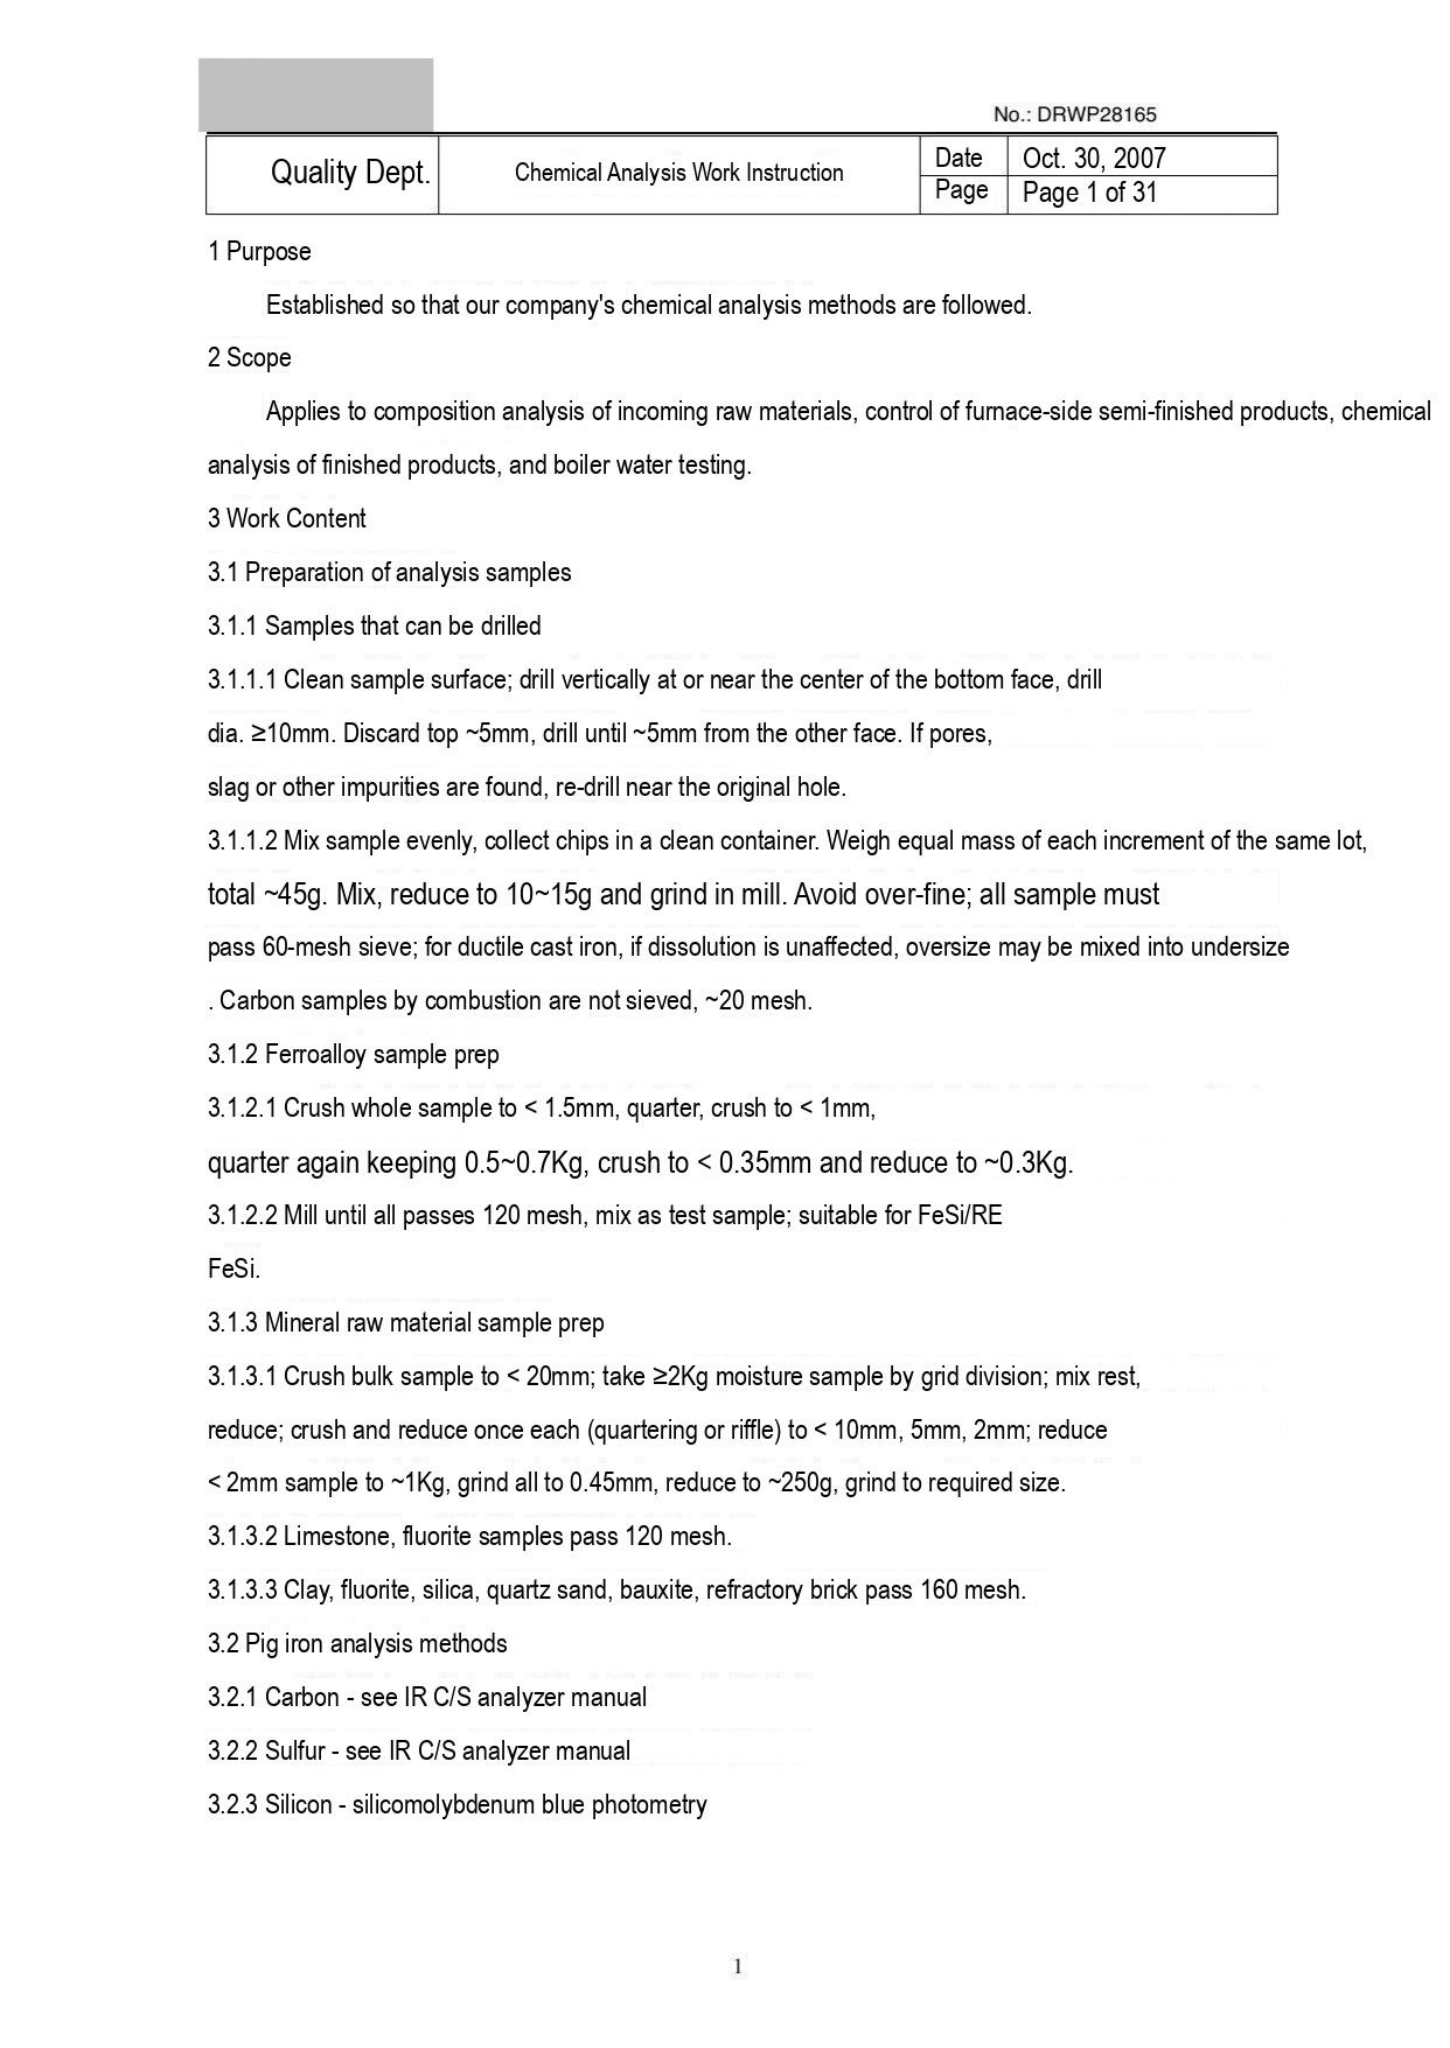No.: DRWP28165

| Quality Dept. | Chemical Analysis Work Instruction | Date | Oct. 30, 2007 |
|---|---|---|---|
| | | Page | Page 1 of 31 |

1 Purpose

Established so that our company's chemical analysis methods are followed.

2 Scope

Applies to composition analysis of incoming raw materials, control of furnace-side semi-finished products, chemical analysis of finished products, and boiler water testing.

3 Work Content

3.1 Preparation of analysis samples

3.1.1 Samples that can be drilled

3.1.1.1 Clean sample surface; drill vertically at or near the center of the bottom face, drill dia. ≥10mm. Discard top ~5mm, drill until ~5mm from the other face. If pores, slag or other impurities are found, re-drill near the original hole.

3.1.1.2 Mix sample evenly, collect chips in a clean container. Weigh equal mass of each increment of the same lot, total ~45g. Mix, reduce to 10~15g and grind in mill. Avoid over-fine; all sample must pass 60-mesh sieve; for ductile cast iron, if dissolution is unaffected, oversize may be mixed into undersize . Carbon samples by combustion are not sieved, ~20 mesh.

3.1.2 Ferroalloy sample prep

3.1.2.1 Crush whole sample to < 1.5mm, quarter, crush to < 1mm, quarter again keeping 0.5~0.7Kg, crush to < 0.35mm and reduce to ~0.3Kg.

3.1.2.2 Mill until all passes 120 mesh, mix as test sample; suitable for FeSi/RE FeSi.

3.1.3 Mineral raw material sample prep

3.1.3.1 Crush bulk sample to < 20mm; take ≥2Kg moisture sample by grid division; mix rest, reduce; crush and reduce once each (quartering or riffle) to < 10mm, 5mm, 2mm; reduce < 2mm sample to ~1Kg, grind all to 0.45mm, reduce to ~250g, grind to required size.

3.1.3.2 Limestone, fluorite samples pass 120 mesh.

3.1.3.3 Clay, fluorite, silica, quartz sand, bauxite, refractory brick pass 160 mesh.

3.2 Pig iron analysis methods

3.2.1 Carbon - see IR C/S analyzer manual

3.2.2 Sulfur - see IR C/S analyzer manual

3.2.3 Silicon - silicomolybdenum blue photometry

1
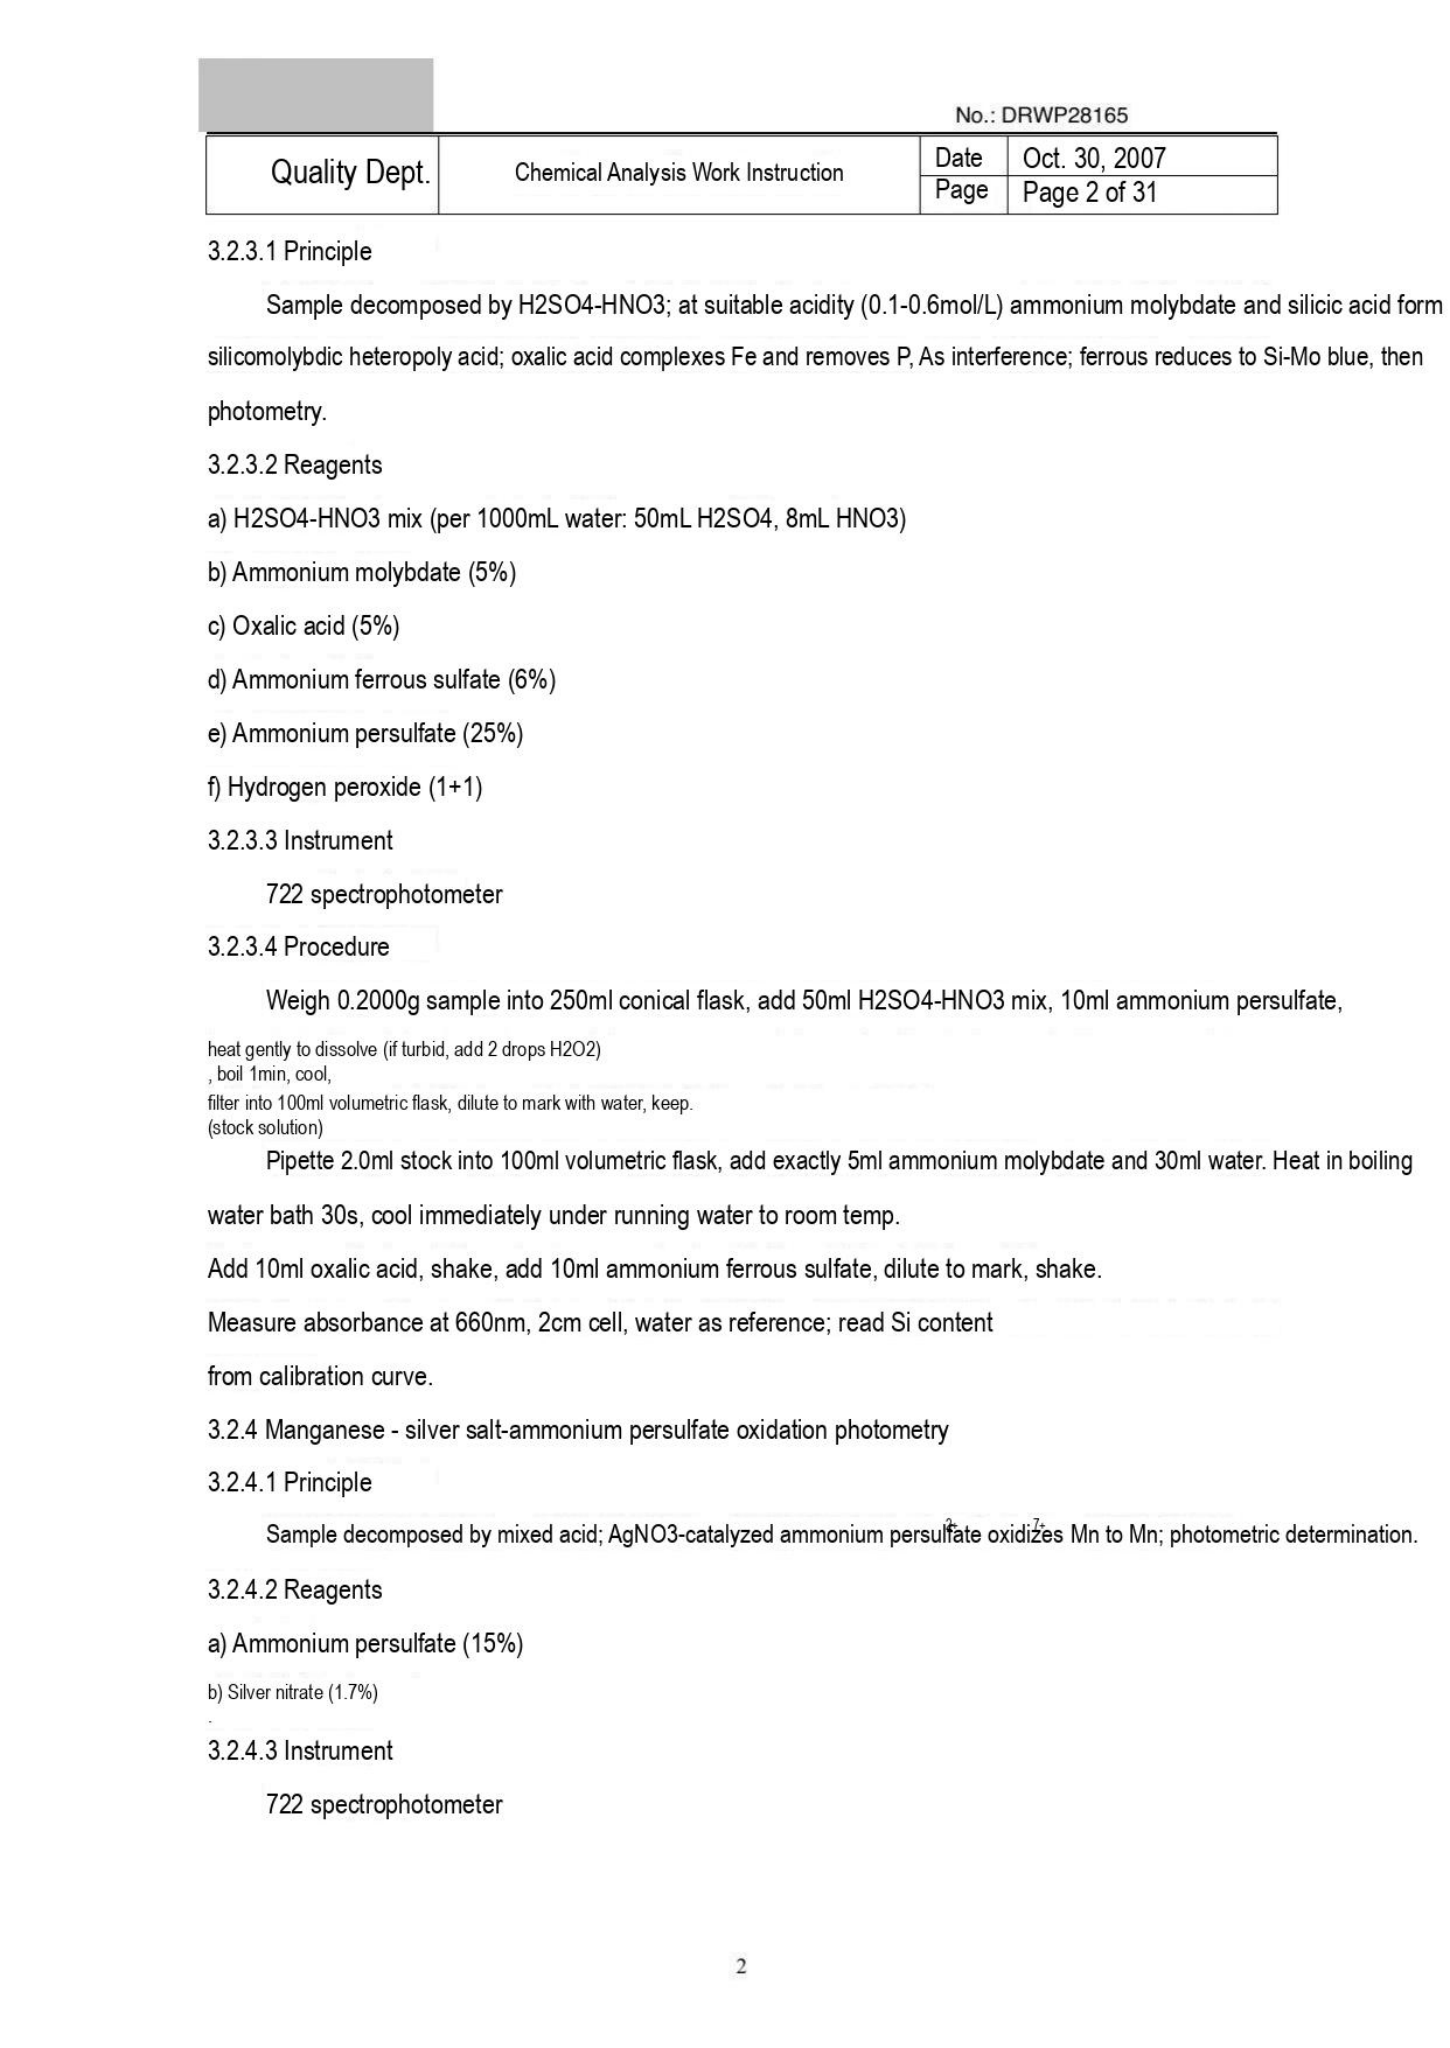No.: DRWP28165

| Quality Dept. | Chemical Analysis Work Instruction | Date | Oct. 30, 2007 |
|---|---|---|---|
| | | Page | Page 2 of 31 |

3.2.3.1 Principle

Sample decomposed by H2SO4-HNO3; at suitable acidity (0.1-0.6mol/L) ammonium molybdate and silicic acid form silicomolybdic heteropoly acid; oxalic acid complexes Fe and removes P, As interference; ferrous reduces to Si-Mo blue, then photometry.

3.2.3.2 Reagents

a) H2SO4-HNO3 mix (per 1000mL water: 50mL H2SO4, 8mL HNO3)

b) Ammonium molybdate (5%)

c) Oxalic acid (5%)

d) Ammonium ferrous sulfate (6%)

e) Ammonium persulfate (25%)

f) Hydrogen peroxide (1+1)

3.2.3.3 Instrument

722 spectrophotometer

3.2.3.4 Procedure

Weigh 0.2000g sample into 250ml conical flask, add 50ml H2SO4-HNO3 mix, 10ml ammonium persulfate,

heat gently to dissolve (if turbid, add 2 drops H2O2)
, boil 1min, cool,
filter into 100ml volumetric flask, dilute to mark with water, keep.
(stock solution)

Pipette 2.0ml stock into 100ml volumetric flask, add exactly 5ml ammonium molybdate and 30ml water. Heat in boiling water bath 30s, cool immediately under running water to room temp.

Add 10ml oxalic acid, shake, add 10ml ammonium ferrous sulfate, dilute to mark, shake.

Measure absorbance at 660nm, 2cm cell, water as reference; read Si content

from calibration curve.

3.2.4 Manganese - silver salt-ammonium persulfate oxidation photometry

3.2.4.1 Principle

Sample decomposed by mixed acid; AgNO3-catalyzed ammonium persulfate oxidizes Mn²⁺ to Mn⁷⁺; photometric determination.

3.2.4.2 Reagents

a) Ammonium persulfate (15%)

b) Silver nitrate (1.7%)

3.2.4.3 Instrument

722 spectrophotometer

2
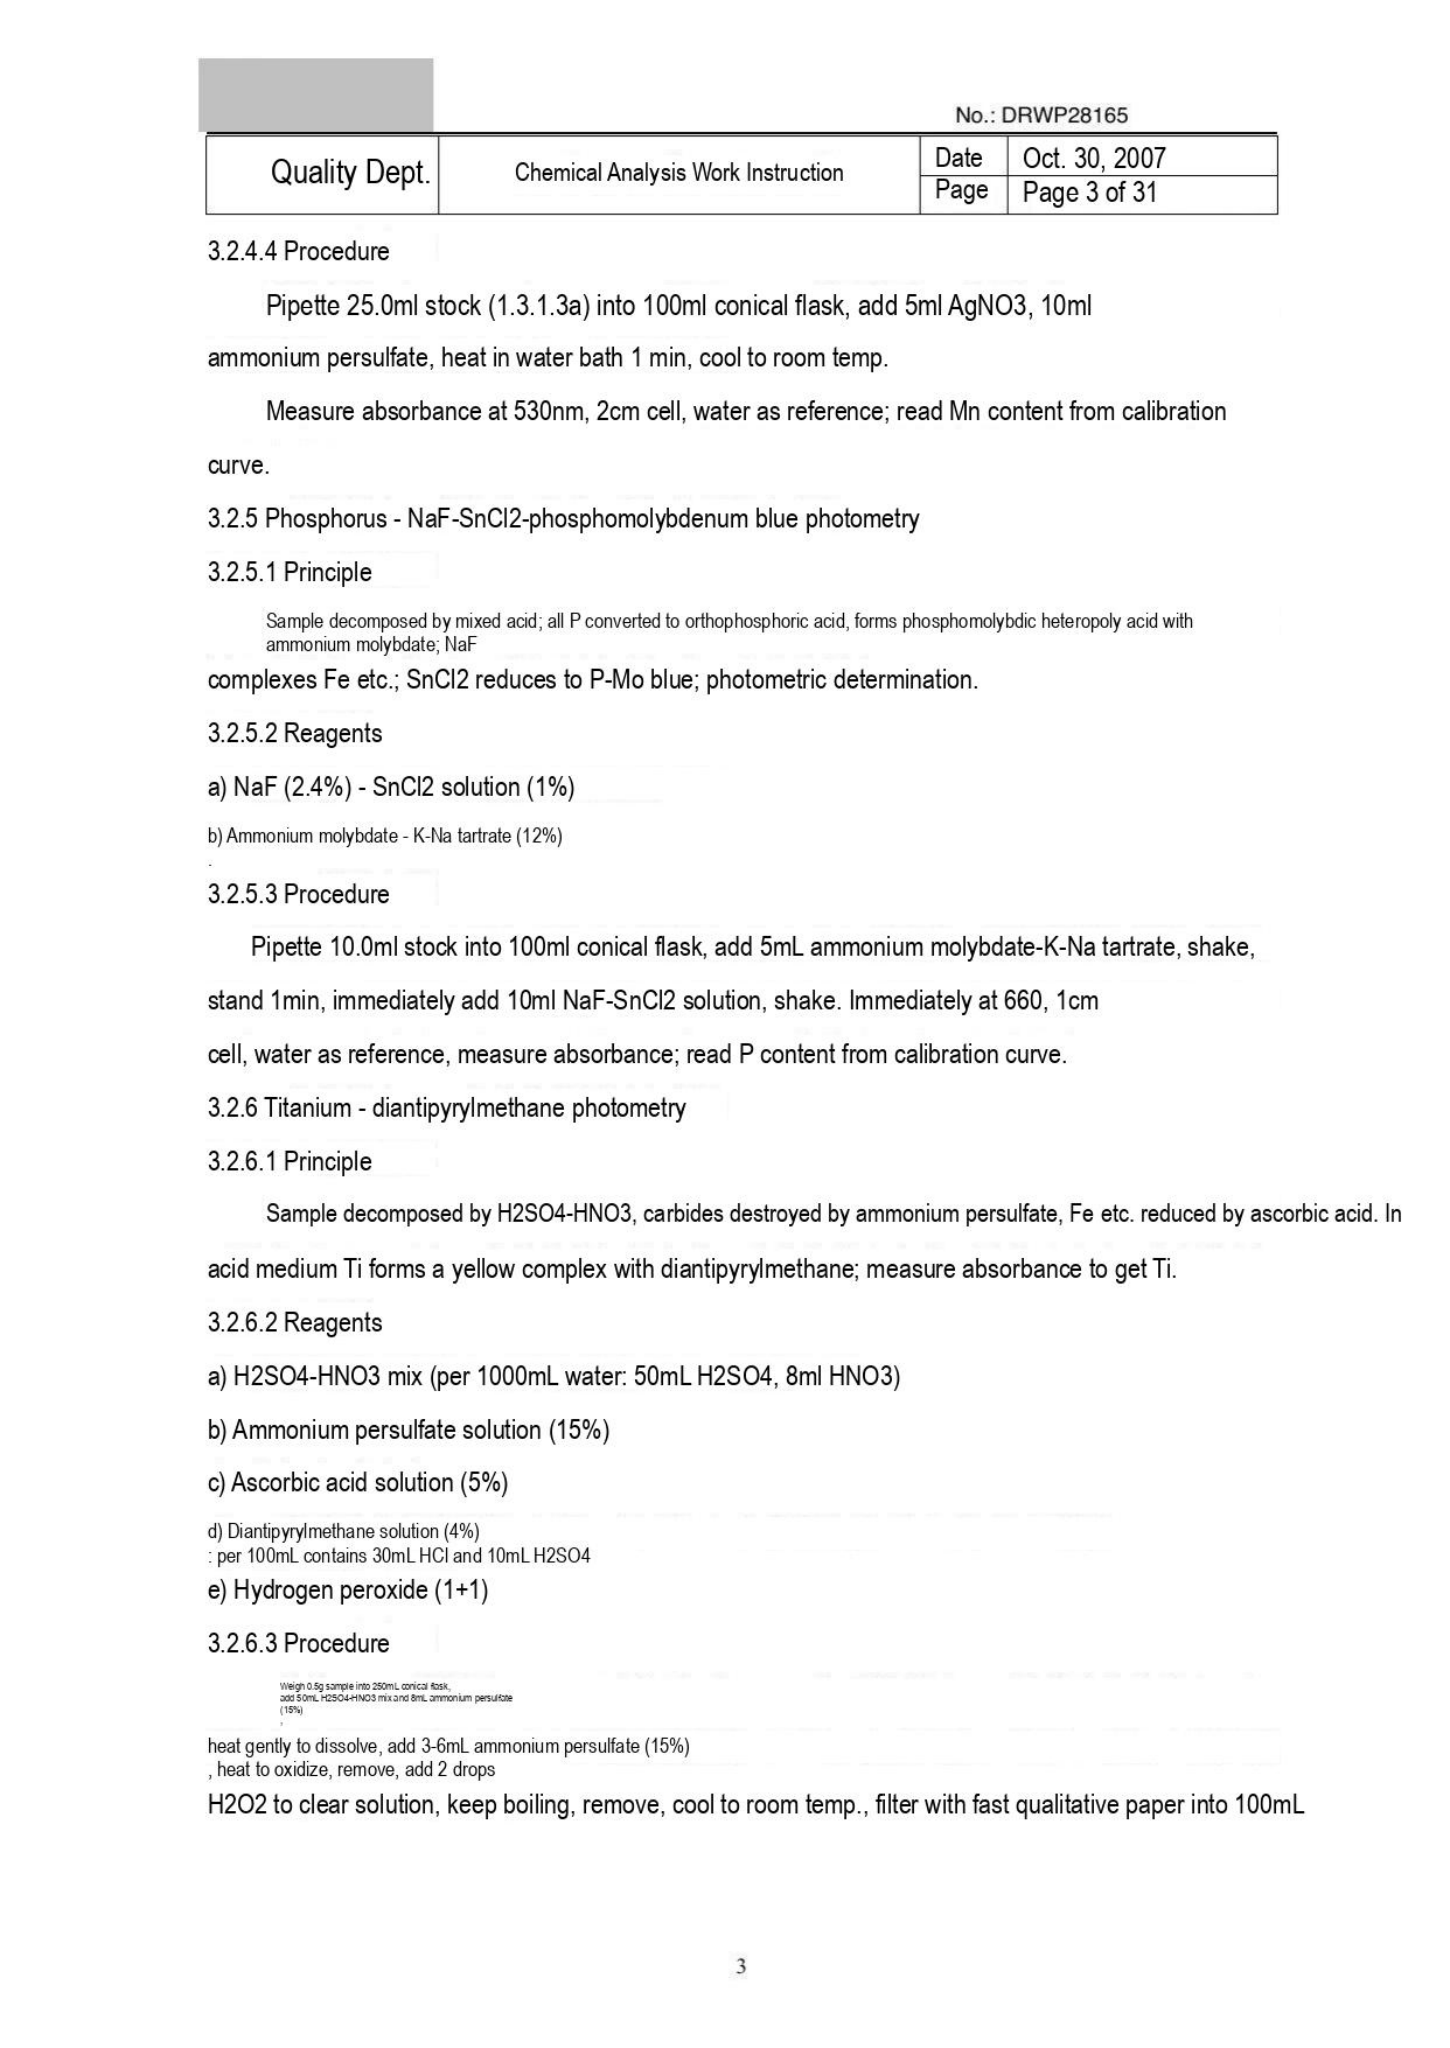No.: DRWP28165

| Quality Dept. | Chemical Analysis Work Instruction | Date | Oct. 30, 2007 |
|---|---|---|---|
| | | Page | Page 3 of 31 |

3.2.4.4 Procedure

Pipette 25.0ml stock (1.3.1.3a) into 100ml conical flask, add 5ml AgNO3, 10ml ammonium persulfate, heat in water bath 1 min, cool to room temp.

Measure absorbance at 530nm, 2cm cell, water as reference; read Mn content from calibration curve.

3.2.5 Phosphorus - NaF-SnCl2-phosphomolybdenum blue photometry

3.2.5.1 Principle

Sample decomposed by mixed acid; all P converted to orthophosphoric acid, forms phosphomolybdic heteropoly acid with ammonium molybdate; NaF complexes Fe etc.; SnCl2 reduces to P-Mo blue; photometric determination.

3.2.5.2 Reagents

a) NaF (2.4%) - SnCl2 solution (1%)

b) Ammonium molybdate - K-Na tartrate (12%)

3.2.5.3 Procedure

Pipette 10.0ml stock into 100ml conical flask, add 5mL ammonium molybdate-K-Na tartrate, shake, stand 1min, immediately add 10ml NaF-SnCl2 solution, shake. Immediately at 660, 1cm cell, water as reference, measure absorbance; read P content from calibration curve.

3.2.6 Titanium - diantipyrylmethane photometry

3.2.6.1 Principle

Sample decomposed by H2SO4-HNO3, carbides destroyed by ammonium persulfate, Fe etc. reduced by ascorbic acid. In acid medium Ti forms a yellow complex with diantipyrylmethane; measure absorbance to get Ti.

3.2.6.2 Reagents

a) H2SO4-HNO3 mix (per 1000mL water: 50mL H2SO4, 8ml HNO3)

b) Ammonium persulfate solution (15%)

c) Ascorbic acid solution (5%)

d) Diantipyrylmethane solution (4%)
: per 100mL contains 30mL HCl and 10mL H2SO4

e) Hydrogen peroxide (1+1)

3.2.6.3 Procedure

Weigh 0.5g sample into 250mL conical flask, add 50mL H2SO4-HNO3 mix and 8mL ammonium persulfate (15%)

heat gently to dissolve, add 3-6mL ammonium persulfate (15%)
, heat to oxidize, remove, add 2 drops
H2O2 to clear solution, keep boiling, remove, cool to room temp., filter with fast qualitative paper into 100mL

3
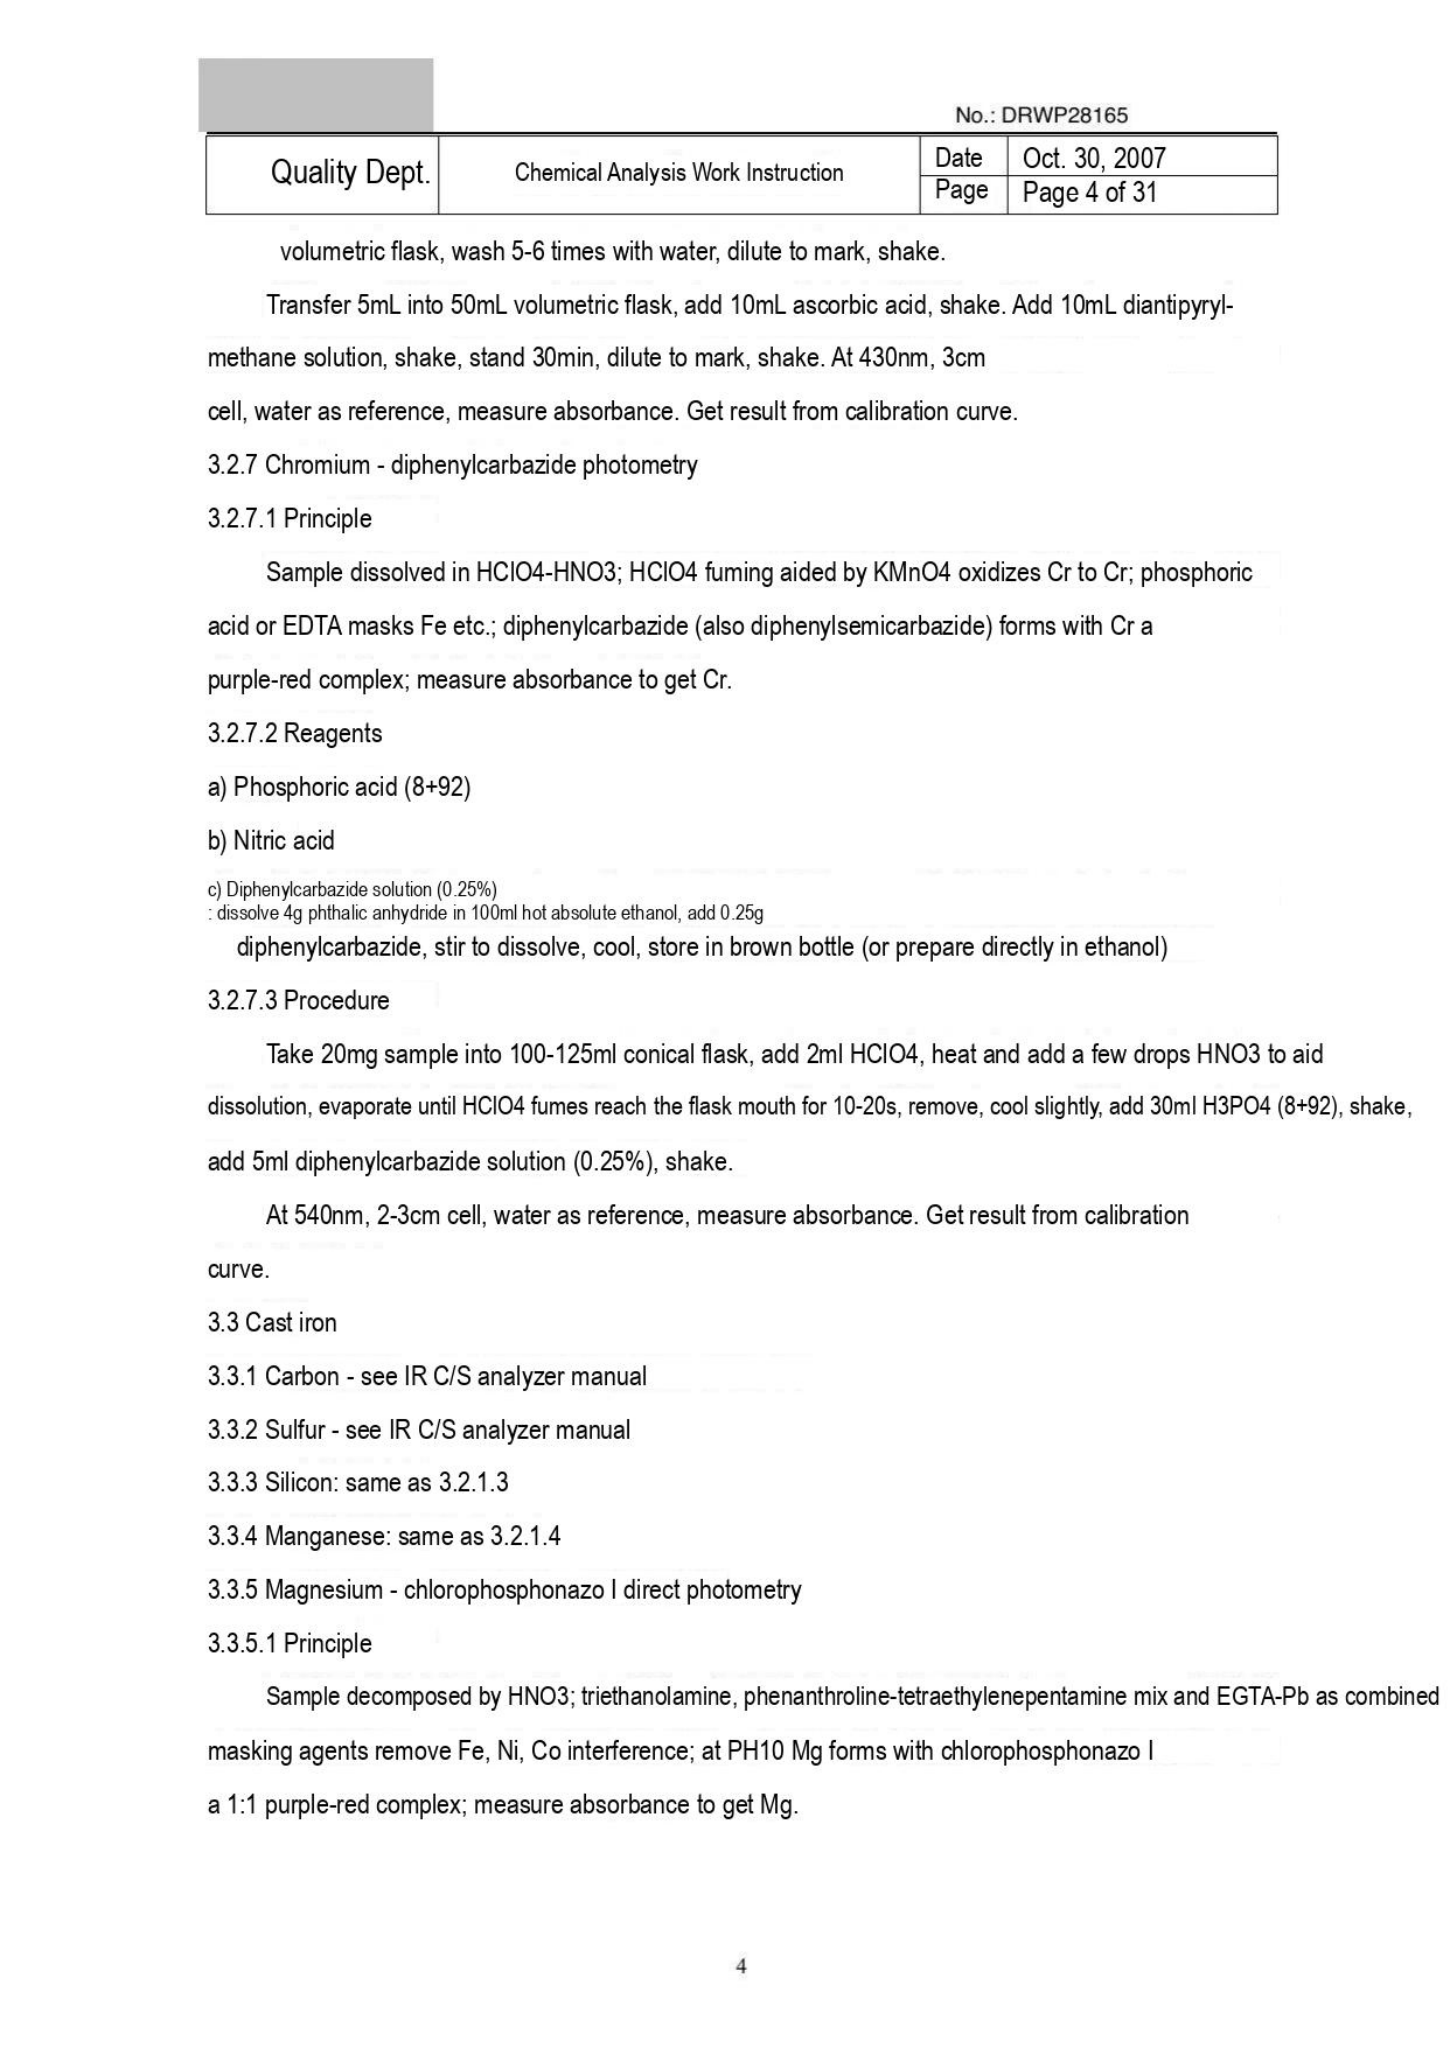No.: DRWP28165

| Quality Dept. | Chemical Analysis Work Instruction | Date | Oct. 30, 2007 |
|---|---|---|---|
| | | Page | Page 4 of 31 |

volumetric flask, wash 5-6 times with water, dilute to mark, shake.

Transfer 5mL into 50mL volumetric flask, add 10mL ascorbic acid, shake. Add 10mL diantipyryl-methane solution, shake, stand 30min, dilute to mark, shake. At 430nm, 3cm cell, water as reference, measure absorbance. Get result from calibration curve.

3.2.7 Chromium - diphenylcarbazide photometry

3.2.7.1 Principle

Sample dissolved in HClO4-HNO3; HClO4 fuming aided by KMnO4 oxidizes Cr to Cr; phosphoric acid or EDTA masks Fe etc.; diphenylcarbazide (also diphenylsemicarbazide) forms with Cr a purple-red complex; measure absorbance to get Cr.

3.2.7.2 Reagents

a) Phosphoric acid (8+92)

b) Nitric acid

c) Diphenylcarbazide solution (0.25%)
: dissolve 4g phthalic anhydride in 100ml hot absolute ethanol, add 0.25g diphenylcarbazide, stir to dissolve, cool, store in brown bottle (or prepare directly in ethanol)

3.2.7.3 Procedure

Take 20mg sample into 100-125ml conical flask, add 2ml HClO4, heat and add a few drops HNO3 to aid dissolution, evaporate until HClO4 fumes reach the flask mouth for 10-20s, remove, cool slightly, add 30ml H3PO4 (8+92), shake, add 5ml diphenylcarbazide solution (0.25%), shake.

At 540nm, 2-3cm cell, water as reference, measure absorbance. Get result from calibration curve.

3.3 Cast iron

3.3.1 Carbon - see IR C/S analyzer manual

3.3.2 Sulfur - see IR C/S analyzer manual

3.3.3 Silicon: same as 3.2.1.3

3.3.4 Manganese: same as 3.2.1.4

3.3.5 Magnesium - chlorophosphonazo I direct photometry

3.3.5.1 Principle

Sample decomposed by HNO3; triethanolamine, phenanthroline-tetraethylenepentamine mix and EGTA-Pb as combined masking agents remove Fe, Ni, Co interference; at PH10 Mg forms with chlorophosphonazo I a 1:1 purple-red complex; measure absorbance to get Mg.

4
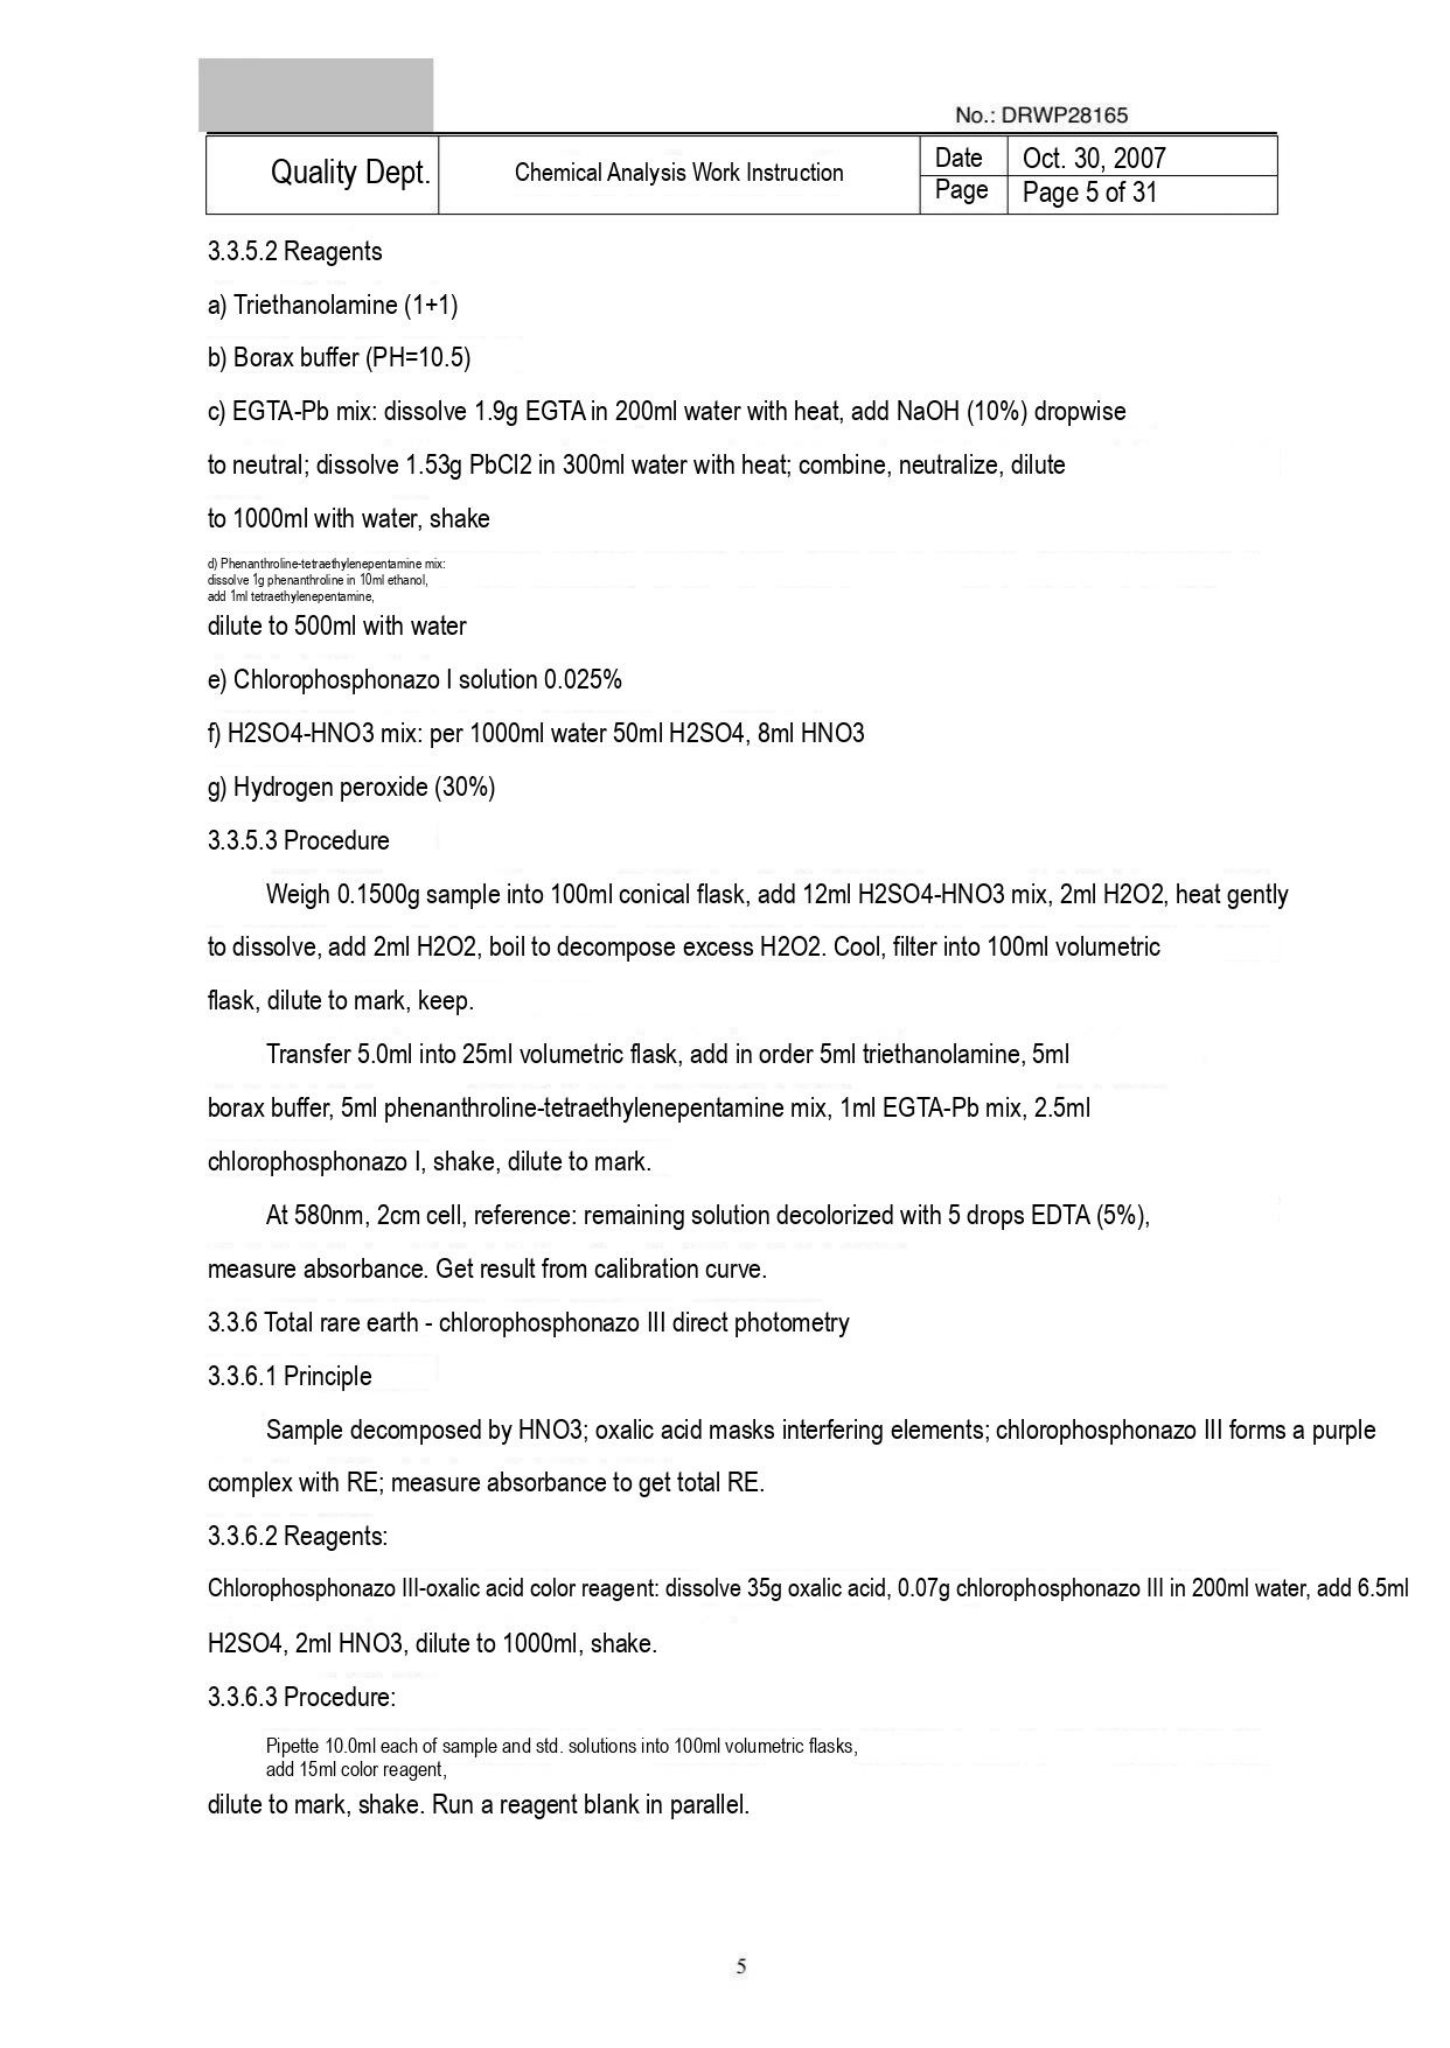No.: DRWP28165

| Quality Dept. | Chemical Analysis Work Instruction | Date | Oct. 30, 2007 |
|---|---|---|---|
| | | Page | Page 5 of 31 |

3.3.5.2 Reagents

a) Triethanolamine (1+1)

b) Borax buffer (PH=10.5)

c) EGTA-Pb mix: dissolve 1.9g EGTA in 200ml water with heat, add NaOH (10%) dropwise to neutral; dissolve 1.53g PbCl2 in 300ml water with heat; combine, neutralize, dilute to 1000ml with water, shake

d) Phenanthroline-tetraethylenepentamine mix: dissolve 1g phenanthroline in 10ml ethanol, add 1ml tetraethylenepentamine, dilute to 500ml with water

e) Chlorophosphonazo I solution 0.025%

f) H2SO4-HNO3 mix: per 1000ml water 50ml H2SO4, 8ml HNO3

g) Hydrogen peroxide (30%)

3.3.5.3 Procedure

Weigh 0.1500g sample into 100ml conical flask, add 12ml H2SO4-HNO3 mix, 2ml H2O2, heat gently to dissolve, add 2ml H2O2, boil to decompose excess H2O2. Cool, filter into 100ml volumetric flask, dilute to mark, keep.

Transfer 5.0ml into 25ml volumetric flask, add in order 5ml triethanolamine, 5ml borax buffer, 5ml phenanthroline-tetraethylenepentamine mix, 1ml EGTA-Pb mix, 2.5ml chlorophosphonazo I, shake, dilute to mark.

At 580nm, 2cm cell, reference: remaining solution decolorized with 5 drops EDTA (5%), measure absorbance. Get result from calibration curve.

3.3.6 Total rare earth - chlorophosphonazo III direct photometry

3.3.6.1 Principle

Sample decomposed by HNO3; oxalic acid masks interfering elements; chlorophosphonazo III forms a purple complex with RE; measure absorbance to get total RE.

3.3.6.2 Reagents:

Chlorophosphonazo III-oxalic acid color reagent: dissolve 35g oxalic acid, 0.07g chlorophosphonazo III in 200ml water, add 6.5ml H2SO4, 2ml HNO3, dilute to 1000ml, shake.

3.3.6.3 Procedure:

Pipette 10.0ml each of sample and std. solutions into 100ml volumetric flasks, add 15ml color reagent, dilute to mark, shake. Run a reagent blank in parallel.

5
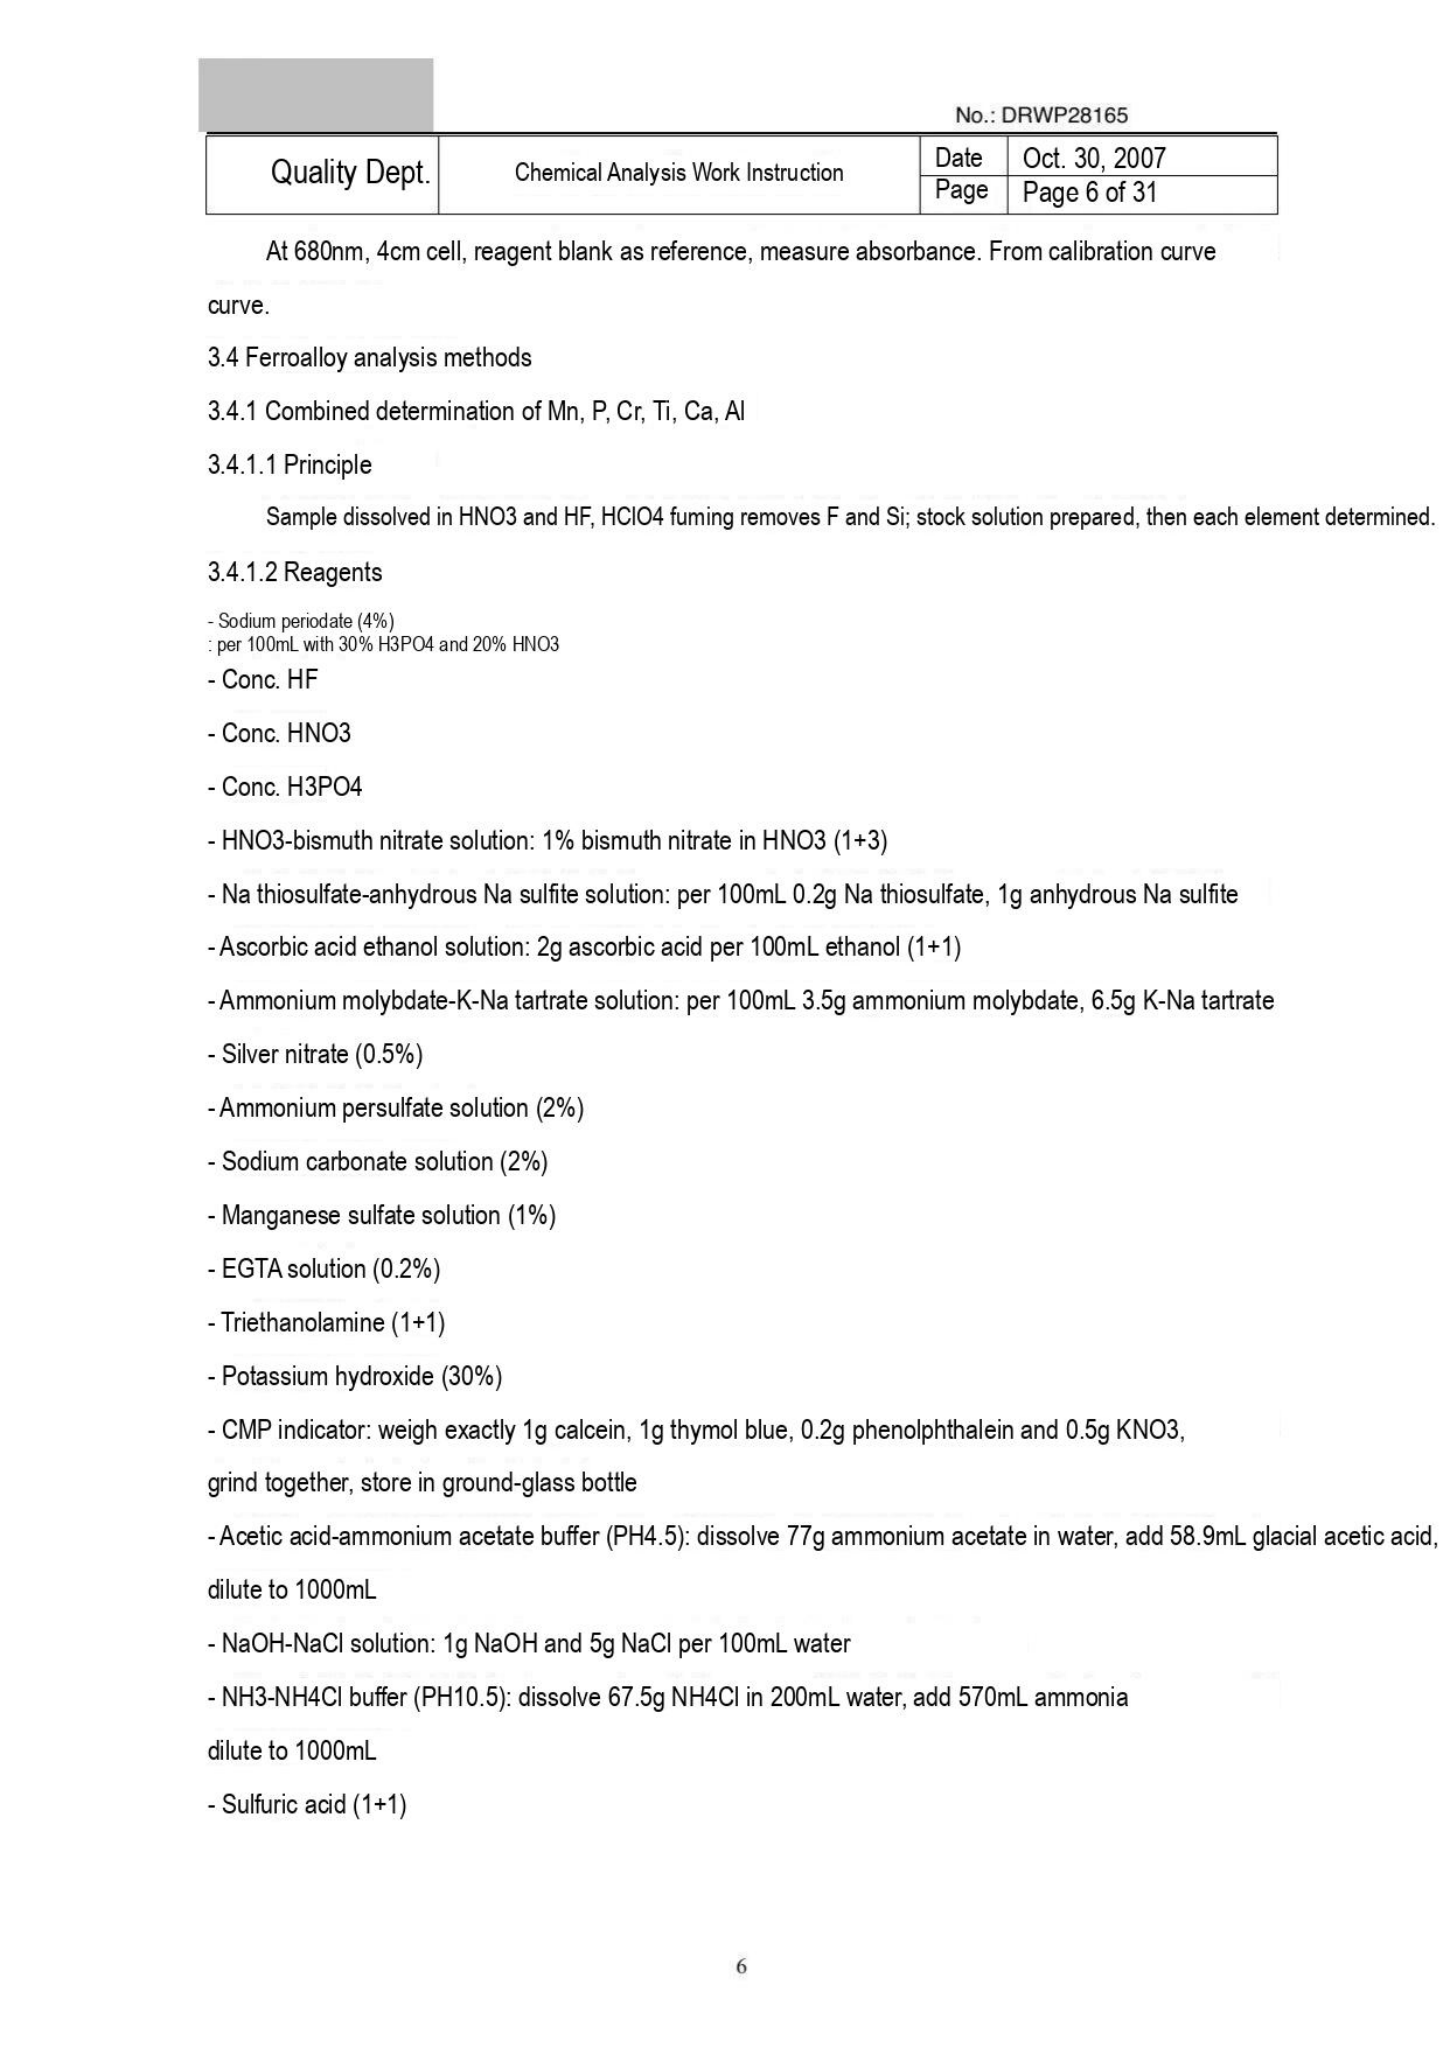No.: DRWP28165

| Quality Dept. | Chemical Analysis Work Instruction | Date | Oct. 30, 2007 |
|---|---|---|---|
| | | Page | Page 6 of 31 |

At 680nm, 4cm cell, reagent blank as reference, measure absorbance. From calibration curve

curve.

3.4 Ferroalloy analysis methods

3.4.1 Combined determination of Mn, P, Cr, Ti, Ca, Al

3.4.1.1 Principle

Sample dissolved in HNO3 and HF, HClO4 fuming removes F and Si; stock solution prepared, then each element determined.

3.4.1.2 Reagents

- Sodium periodate (4%)
: per 100mL with 30% H3PO4 and 20% HNO3

- Conc. HF

- Conc. HNO3

- Conc. H3PO4

- HNO3-bismuth nitrate solution: 1% bismuth nitrate in HNO3 (1+3)

- Na thiosulfate-anhydrous Na sulfite solution: per 100mL 0.2g Na thiosulfate, 1g anhydrous Na sulfite

- Ascorbic acid ethanol solution: 2g ascorbic acid per 100mL ethanol (1+1)

- Ammonium molybdate-K-Na tartrate solution: per 100mL 3.5g ammonium molybdate, 6.5g K-Na tartrate

- Silver nitrate (0.5%)

- Ammonium persulfate solution (2%)

- Sodium carbonate solution (2%)

- Manganese sulfate solution (1%)

- EGTA solution (0.2%)

- Triethanolamine (1+1)

- Potassium hydroxide (30%)

- CMP indicator: weigh exactly 1g calcein, 1g thymol blue, 0.2g phenolphthalein and 0.5g KNO3,

grind together, store in ground-glass bottle

- Acetic acid-ammonium acetate buffer (PH4.5): dissolve 77g ammonium acetate in water, add 58.9mL glacial acetic acid,

dilute to 1000mL

- NaOH-NaCl solution: 1g NaOH and 5g NaCl per 100mL water

- NH3-NH4Cl buffer (PH10.5): dissolve 67.5g NH4Cl in 200mL water, add 570mL ammonia

dilute to 1000mL

- Sulfuric acid (1+1)

6